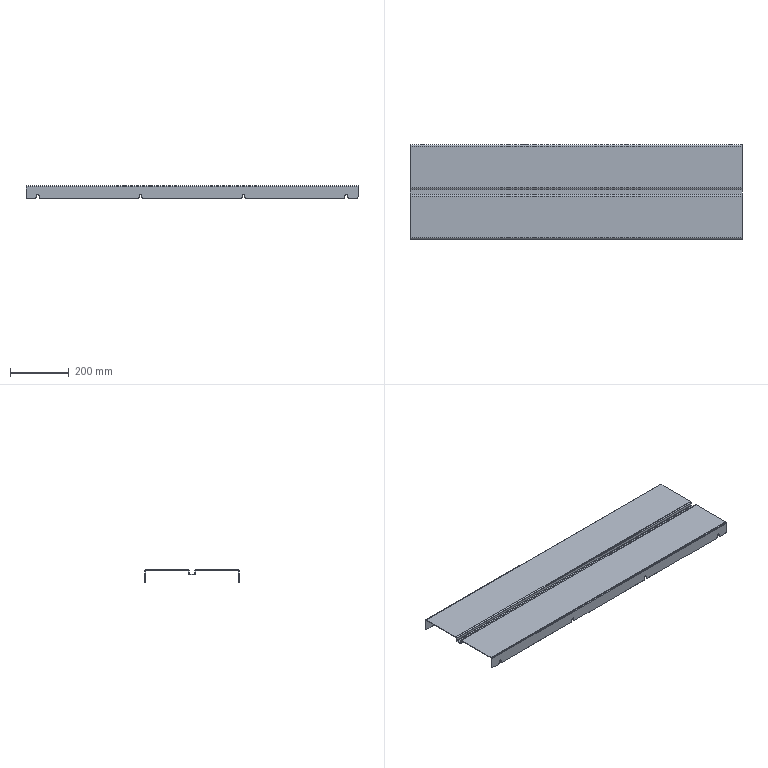Part | STEP file | BELT.PLATE.1.stp | 1 solid | 90 faces | box 1130 x 320 x 43 mm | volume 956827 mm3 | spline 42 | cylinder 28 | plane 20 | commonest cylinder face diameters 10 x12 4 x6 8 x6 9 x4